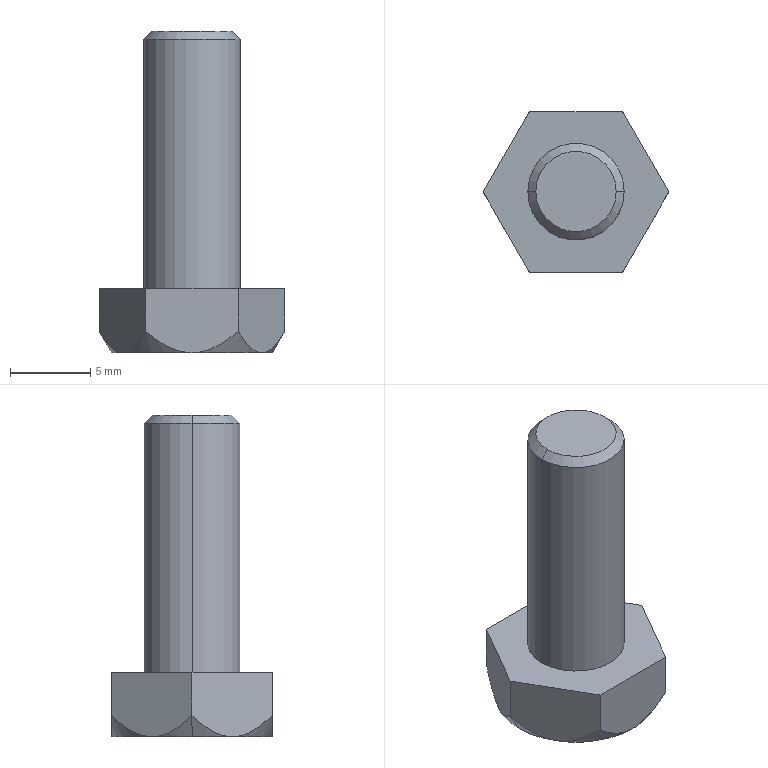Part | SolidWorks | features ICE 2, Chamfer 1, Extrusion 1 | 1 solid | 20 faces | box 11.547 x 10 x 20 mm | volume 793.318 mm3 | cone 9 | plane 9 | cylinder 2 | commonest cylinder face diameters 6 x2
STEP:
#1=CARTESIAN_POINT('',(2.5,0.,20.));
#2=VERTEX_POINT('',#1);
#3=CARTESIAN_POINT('',(-2.5,0.,20.));
#4=VERTEX_POINT('',#3);
#5=CARTESIAN_POINT('',(0.,0.,20.));
#6=DIRECTION('',(0.,0.,1.));
#7=DIRECTION('',(1.,0.,0.));
#8=AXIS2_PLACEMENT_3D('',#5,#6,#7);
#9=CIRCLE('',#8,2.5);
#10=EDGE_CURVE('',#2,#4,#9,.T.);
#11=ORIENTED_EDGE('',*,*,#10,.F.);
#12=CARTESIAN_POINT('',(3.,0.,19.5));
#13=VERTEX_POINT('',#12);
#14=CARTESIAN_POINT('',(2.5,0.,20.));
#15=DIRECTION('',(0.7071,0.,-0.7071));
#16=VECTOR('',#15,1000.);
#17=LINE('',#14,#16);
#18=EDGE_CURVE('',#2,#13,#17,.T.);
#19=ORIENTED_EDGE('',*,*,#18,.T.);
#20=CARTESIAN_POINT('',(-3.,0.,19.5));
#21=VERTEX_POINT('',#20);
#22=CARTESIAN_POINT('',(0.,0.,19.5));
#23=DIRECTION('',(0.,0.,-1.));
#24=DIRECTION('',(1.,0.,0.));
#25=AXIS2_PLACEMENT_3D('',#22,#23,#24);
#26=CIRCLE('',#25,3.);
#27=EDGE_CURVE('',#21,#13,#26,.T.);
#28=ORIENTED_EDGE('',*,*,#27,.F.);
#29=CARTESIAN_POINT('',(-2.5,0.,20.));
#30=DIRECTION('',(-0.7071,0.,-0.7071));
#31=VECTOR('',#30,1000.);
#32=LINE('',#29,#31);
#33=EDGE_CURVE('',#4,#21,#32,.T.);
#34=ORIENTED_EDGE('',*,*,#33,.F.);
#35=EDGE_LOOP('',(#11,#19,#28,#34));
#36=FACE_OUTER_BOUND('',#35,.T.);
#37=CARTESIAN_POINT('',(0.,0.,20.));
#38=DIRECTION('',(0.,0.,-1.));
#39=DIRECTION('',(-1.,0.,0.));
#40=AXIS2_PLACEMENT_3D('',#37,#38,#39);
#41=CONICAL_SURFACE('',#40,2.5,0.7854);
#42=ADVANCED_FACE('',(#36),#41,.T.);
#43=ORIENTED_EDGE('',*,*,#27,.T.);
#44=CARTESIAN_POINT('',(3.,0.,4.));
#45=VERTEX_POINT('',#44);
#46=CARTESIAN_POINT('',(3.,0.,20.));
#47=DIRECTION('',(0.,0.,-1.));
#48=VECTOR('',#47,1000.);
#49=LINE('',#46,#48);
#50=EDGE_CURVE('',#13,#45,#49,.T.);
#51=ORIENTED_EDGE('',*,*,#50,.T.);
#52=CARTESIAN_POINT('',(-3.,0.,4.));
#53=VERTEX_POINT('',#52);
#54=CARTESIAN_POINT('',(0.,0.,4.));
#55=DIRECTION('',(0.,0.,1.));
#56=DIRECTION('',(1.,0.,0.));
#57=AXIS2_PLACEMENT_3D('',#54,#55,#56);
#58=CIRCLE('',#57,3.);
#59=EDGE_CURVE('',#45,#53,#58,.T.);
#60=ORIENTED_EDGE('',*,*,#59,.T.);
#61=CARTESIAN_POINT('',(-3.,0.,20.));
#62=DIRECTION('',(0.,0.,-1.));
#63=VECTOR('',#62,1000.);
#64=LINE('',#61,#63);
#65=EDGE_CURVE('',#21,#53,#64,.T.);
#66=ORIENTED_EDGE('',*,*,#65,.F.);
#67=EDGE_LOOP('',(#43,#51,#60,#66));
#68=FACE_OUTER_BOUND('',#67,.T.);
#69=CARTESIAN_POINT('',(0.,0.,20.));
#70=DIRECTION('',(0.,0.,-1.));
#71=DIRECTION('',(-1.,0.,0.));
#72=AXIS2_PLACEMENT_3D('',#69,#70,#71);
#73=CYLINDRICAL_SURFACE('',#72,3.);
#74=ADVANCED_FACE('',(#68),#73,.T.);
#75=CARTESIAN_POINT('',(-4.33,2.5,0.));
#76=VERTEX_POINT('',#75);
#77=CARTESIAN_POINT('',(-5.,0.,0.));
#78=VERTEX_POINT('',#77);
#79=CARTESIAN_POINT('',(0.,0.,0.));
#80=DIRECTION('',(0.,0.,1.));
#81=DIRECTION('',(1.,0.,0.));
#82=AXIS2_PLACEMENT_3D('',#79,#80,#81);
#83=CIRCLE('',#82,5.);
#84=EDGE_CURVE('',#76,#78,#83,.T.);
#85=ORIENTED_EDGE('',*,*,#84,.T.);
#86=CARTESIAN_POINT('',(-5.774,0.,1.34));
#87=VERTEX_POINT('',#86);
#88=CARTESIAN_POINT('',(-5.,0.,0.));
#89=DIRECTION('',(-0.5,0.,0.866));
#90=VECTOR('',#89,1000.);
#91=LINE('',#88,#90);
#92=EDGE_CURVE('',#78,#87,#91,.T.);
#93=ORIENTED_EDGE('',*,*,#92,.T.);
#94=CARTESIAN_POINT('',(-5.774,0.,1.34));
#95=CARTESIAN_POINT('',(-5.568,0.3557,0.9841));
#96=CARTESIAN_POINT('',(-5.352,0.7302,0.6615));
#97=CARTESIAN_POINT('',(-4.991,1.355,0.2887));
#98=CARTESIAN_POINT('',(-4.864,1.576,0.1837));
#99=CARTESIAN_POINT('',(-4.668,1.915,0.07581));
#100=CARTESIAN_POINT('',(-4.602,2.03,0.0478));
#101=CARTESIAN_POINT('',(-4.467,2.263,0.009812));
#102=CARTESIAN_POINT('',(-4.398,2.383,0.));
#103=CARTESIAN_POINT('',(-4.33,2.5,0.));
#104=B_SPLINE_CURVE_WITH_KNOTS('',3,(#94,#95,#96,#97,#98,#99,#100,#101,#102,#103),.UNSPECIFIED.,.F.,.F.,(4,2,2,2,4),(0.000000303,0.001616,0.002424,0.002828,0.003232),.UNSPECIFIED.);
#105=EDGE_CURVE('',#87,#76,#104,.T.);
#106=ORIENTED_EDGE('',*,*,#105,.T.);
#107=EDGE_LOOP('',(#85,#93,#106));
#108=FACE_OUTER_BOUND('',#107,.T.);
#109=CARTESIAN_POINT('',(0.,0.,0.));
#110=DIRECTION('',(0.,0.,1.));
#111=DIRECTION('',(-1.,0.,0.));
#112=AXIS2_PLACEMENT_3D('',#109,#110,#111);
#113=CONICAL_SURFACE('',#112,5.,0.5236);
#114=ADVANCED_FACE('',(#108),#113,.T.);
#115=CARTESIAN_POINT('',(2.887,5.,1.34));
#116=VERTEX_POINT('',#115);
#117=CARTESIAN_POINT('',(4.33,2.5,0.));
#118=VERTEX_POINT('',#117);
#119=CARTESIAN_POINT('',(2.887,5.,1.34));
#120=CARTESIAN_POINT('',(3.092,4.644,0.9841));
#121=CARTESIAN_POINT('',(3.308,4.27,0.6615));
#122=CARTESIAN_POINT('',(3.669,3.645,0.2887));
#123=CARTESIAN_POINT('',(3.797,3.424,0.1837));
#124=CARTESIAN_POINT('',(3.992,3.085,0.07581));
#125=CARTESIAN_POINT('',(4.059,2.97,0.0478));
#126=CARTESIAN_POINT('',(4.193,2.737,0.009812));
#127=CARTESIAN_POINT('',(4.262,2.617,0.));
#128=CARTESIAN_POINT('',(4.33,2.5,0.));
#129=B_SPLINE_CURVE_WITH_KNOTS('',3,(#119,#120,#121,#122,#123,#124,#125,#126,#127,#128),.UNSPECIFIED.,.F.,.F.,(4,2,2,2,4),(0.000000303,0.001616,0.002424,0.002828,0.003232),.UNSPECIFIED.);
#130=EDGE_CURVE('',#116,#118,#129,.T.);
#131=ORIENTED_EDGE('',*,*,#130,.F.);
#132=CARTESIAN_POINT('',(2.887,5.,4.));
#133=VERTEX_POINT('',#132);
#134=CARTESIAN_POINT('',(2.887,5.,4.));
#135=DIRECTION('',(0.,0.,-1.));
#136=VECTOR('',#135,1000.);
#137=LINE('',#134,#136);
#138=EDGE_CURVE('',#133,#116,#137,.T.);
#139=ORIENTED_EDGE('',*,*,#138,.F.);
#140=CARTESIAN_POINT('',(5.774,0.,4.));
#141=VERTEX_POINT('',#140);
#142=CARTESIAN_POINT('',(5.774,0.,4.));
#143=DIRECTION('',(-0.5,0.866,0.));
#144=VECTOR('',#143,1000.);
#145=LINE('',#142,#144);
#146=EDGE_CURVE('',#141,#133,#145,.T.);
#147=ORIENTED_EDGE('',*,*,#146,.F.);
#148=CARTESIAN_POINT('',(5.774,0.,1.34));
#149=VERTEX_POINT('',#148);
#150=CARTESIAN_POINT('',(5.774,0.,4.));
#151=DIRECTION('',(0.,0.,-1.));
#152=VECTOR('',#151,1000.);
#153=LINE('',#150,#152);
#154=EDGE_CURVE('',#141,#149,#153,.T.);
#155=ORIENTED_EDGE('',*,*,#154,.T.);
#156=CARTESIAN_POINT('',(4.33,2.5,0.));
#157=CARTESIAN_POINT('',(4.466,2.265,0.));
#158=CARTESIAN_POINT('',(4.599,2.034,0.0383));
#159=CARTESIAN_POINT('',(4.863,1.578,0.1827));
#160=CARTESIAN_POINT('',(4.988,1.361,0.2859));
#161=CARTESIAN_POINT('',(5.228,0.9455,0.5326));
#162=CARTESIAN_POINT('',(5.343,0.7456,0.6772));
#163=CARTESIAN_POINT('',(5.565,0.3618,0.9919));
#164=CARTESIAN_POINT('',(5.671,0.1781,1.162));
#165=CARTESIAN_POINT('',(5.774,0.,1.34));
#166=B_SPLINE_CURVE_WITH_KNOTS('',3,(#156,#157,#158,#159,#160,#161,#162,#163,#164,#165),.UNSPECIFIED.,.F.,.F.,(4,2,2,2,4),(0.003232,0.004038,0.004845,0.005652,0.006458),.UNSPECIFIED.);
#167=EDGE_CURVE('',#118,#149,#166,.T.);
#168=ORIENTED_EDGE('',*,*,#167,.F.);
#169=EDGE_LOOP('',(#131,#139,#147,#155,#168));
#170=FACE_OUTER_BOUND('',#169,.T.);
#171=CARTESIAN_POINT('',(5.774,0.,4.));
#172=DIRECTION('',(-0.866,-0.5,0.));
#173=DIRECTION('',(0.5,-0.866,0.));
#174=AXIS2_PLACEMENT_3D('',#171,#172,#173);
#175=PLANE('',#174);
#176=ADVANCED_FACE('',(#170),#175,.F.);
#177=CARTESIAN_POINT('',(-2.887,5.,1.34));
#178=VERTEX_POINT('',#177);
#179=CARTESIAN_POINT('',(0.,5.,0.));
#180=VERTEX_POINT('',#179);
#181=CARTESIAN_POINT('',(-2.887,5.,1.34));
#182=CARTESIAN_POINT('',(-2.683,5.,1.163));
#183=CARTESIAN_POINT('',(-2.472,5.,0.9945));
#184=CARTESIAN_POINT('',(-2.031,5.,0.6804));
#185=CARTESIAN_POINT('',(-1.798,5.,0.5344));
#186=CARTESIAN_POINT('',(-1.316,5.,0.286));
#187=CARTESIAN_POINT('',(-1.063,5.,0.1822));
#188=CARTESIAN_POINT('',(-0.5366,5.,0.03808));
#189=CARTESIAN_POINT('',(-0.2701,5.,0.));
#190=CARTESIAN_POINT('',(0.,5.,0.));
#191=B_SPLINE_CURVE_WITH_KNOTS('',3,(#181,#182,#183,#184,#185,#186,#187,#188,#189,#190),.UNSPECIFIED.,.F.,.F.,(4,2,2,2,4),(0.01162,0.01244,0.01325,0.01406,0.01487),.UNSPECIFIED.);
#192=EDGE_CURVE('',#178,#180,#191,.T.);
#193=ORIENTED_EDGE('',*,*,#192,.F.);
#194=CARTESIAN_POINT('',(-2.887,5.,4.));
#195=VERTEX_POINT('',#194);
#196=CARTESIAN_POINT('',(-2.887,5.,4.));
#197=DIRECTION('',(0.,0.,-1.));
#198=VECTOR('',#197,1000.);
#199=LINE('',#196,#198);
#200=EDGE_CURVE('',#195,#178,#199,.T.);
#201=ORIENTED_EDGE('',*,*,#200,.F.);
#202=CARTESIAN_POINT('',(2.887,5.,4.));
#203=DIRECTION('',(-1.,0.,0.));
#204=VECTOR('',#203,1000.);
#205=LINE('',#202,#204);
#206=EDGE_CURVE('',#133,#195,#205,.T.);
#207=ORIENTED_EDGE('',*,*,#206,.F.);
#208=ORIENTED_EDGE('',*,*,#138,.T.);
#209=CARTESIAN_POINT('',(0.,5.,0.));
#210=CARTESIAN_POINT('',(0.2696,5.,0.));
#211=CARTESIAN_POINT('',(0.5439,5.,0.03965));
#212=CARTESIAN_POINT('',(1.066,5.,0.1833));
#213=CARTESIAN_POINT('',(1.32,5.,0.2879));
#214=CARTESIAN_POINT('',(2.042,5.,0.6607));
#215=CARTESIAN_POINT('',(2.477,5.,0.9847));
#216=CARTESIAN_POINT('',(2.887,5.,1.34));
#217=B_SPLINE_CURVE_WITH_KNOTS('',3,(#209,#210,#211,#212,#213,#214,#215,#216),.UNSPECIFIED.,.F.,.F.,(4,2,2,4),(0.01487,0.01568,0.01649,0.01812),.UNSPECIFIED.);
#218=EDGE_CURVE('',#180,#116,#217,.T.);
#219=ORIENTED_EDGE('',*,*,#218,.F.);
#220=EDGE_LOOP('',(#193,#201,#207,#208,#219));
#221=FACE_OUTER_BOUND('',#220,.T.);
#222=CARTESIAN_POINT('',(2.887,5.,4.));
#223=DIRECTION('',(0.,-1.,0.));
#224=DIRECTION('',(1.,0.,0.));
#225=AXIS2_PLACEMENT_3D('',#222,#223,#224);
#226=PLANE('',#225);
#227=ADVANCED_FACE('',(#221),#226,.F.);
#228=ORIENTED_EDGE('',*,*,#105,.F.);
#229=CARTESIAN_POINT('',(-5.774,0.,4.));
#230=VERTEX_POINT('',#229);
#231=CARTESIAN_POINT('',(-5.774,0.,4.));
#232=DIRECTION('',(0.,0.,-1.));
#233=VECTOR('',#232,1000.);
#234=LINE('',#231,#233);
#235=EDGE_CURVE('',#230,#87,#234,.T.);
#236=ORIENTED_EDGE('',*,*,#235,.F.);
#237=CARTESIAN_POINT('',(-2.887,5.,4.));
#238=DIRECTION('',(-0.5,-0.866,0.));
#239=VECTOR('',#238,1000.);
#240=LINE('',#237,#239);
#241=EDGE_CURVE('',#195,#230,#240,.T.);
#242=ORIENTED_EDGE('',*,*,#241,.F.);
#243=ORIENTED_EDGE('',*,*,#200,.T.);
#244=CARTESIAN_POINT('',(-4.33,2.5,0.));
#245=CARTESIAN_POINT('',(-4.195,2.735,0.));
#246=CARTESIAN_POINT('',(-4.061,2.966,0.0383));
#247=CARTESIAN_POINT('',(-3.798,3.422,0.1827));
#248=CARTESIAN_POINT('',(-3.672,3.639,0.2859));
#249=CARTESIAN_POINT('',(-3.433,4.055,0.5326));
#250=CARTESIAN_POINT('',(-3.317,4.254,0.6772));
#251=CARTESIAN_POINT('',(-3.096,4.638,0.9919));
#252=CARTESIAN_POINT('',(-2.99,4.822,1.162));
#253=CARTESIAN_POINT('',(-2.887,5.,1.34));
#254=B_SPLINE_CURVE_WITH_KNOTS('',3,(#244,#245,#246,#247,#248,#249,#250,#251,#252,#253),.UNSPECIFIED.,.F.,.F.,(4,2,2,2,4),(0.003232,0.004038,0.004845,0.005652,0.006458),.UNSPECIFIED.);
#255=EDGE_CURVE('',#76,#178,#254,.T.);
#256=ORIENTED_EDGE('',*,*,#255,.F.);
#257=EDGE_LOOP('',(#228,#236,#242,#243,#256));
#258=FACE_OUTER_BOUND('',#257,.T.);
#259=CARTESIAN_POINT('',(-2.887,5.,4.));
#260=DIRECTION('',(0.866,-0.5,0.));
#261=DIRECTION('',(0.5,0.866,0.));
#262=AXIS2_PLACEMENT_3D('',#259,#260,#261);
#263=PLANE('',#262);
#264=ADVANCED_FACE('',(#258),#263,.F.);
#265=CARTESIAN_POINT('',(-2.887,-5.,1.34));
#266=VERTEX_POINT('',#265);
#267=CARTESIAN_POINT('',(-4.33,-2.5,0.));
#268=VERTEX_POINT('',#267);
#269=CARTESIAN_POINT('',(-2.887,-5.,1.34));
#270=CARTESIAN_POINT('',(-3.092,-4.644,0.9841));
#271=CARTESIAN_POINT('',(-3.308,-4.27,0.6615));
#272=CARTESIAN_POINT('',(-3.669,-3.645,0.2887));
#273=CARTESIAN_POINT('',(-3.797,-3.424,0.1837));
#274=CARTESIAN_POINT('',(-3.992,-3.085,0.07581));
#275=CARTESIAN_POINT('',(-4.059,-2.97,0.0478));
#276=CARTESIAN_POINT('',(-4.193,-2.737,0.009812));
#277=CARTESIAN_POINT('',(-4.262,-2.617,0.));
#278=CARTESIAN_POINT('',(-4.33,-2.5,0.));
#279=B_SPLINE_CURVE_WITH_KNOTS('',3,(#269,#270,#271,#272,#273,#274,#275,#276,#277,#278),.UNSPECIFIED.,.F.,.F.,(4,2,2,2,4),(0.000000303,0.001616,0.002424,0.002828,0.003232),.UNSPECIFIED.);
#280=EDGE_CURVE('',#266,#268,#279,.T.);
#281=ORIENTED_EDGE('',*,*,#280,.F.);
#282=CARTESIAN_POINT('',(-2.887,-5.,4.));
#283=VERTEX_POINT('',#282);
#284=CARTESIAN_POINT('',(-2.887,-5.,4.));
#285=DIRECTION('',(0.,0.,-1.));
#286=VECTOR('',#285,1000.);
#287=LINE('',#284,#286);
#288=EDGE_CURVE('',#283,#266,#287,.T.);
#289=ORIENTED_EDGE('',*,*,#288,.F.);
#290=CARTESIAN_POINT('',(-5.774,0.,4.));
#291=DIRECTION('',(0.5,-0.866,0.));
#292=VECTOR('',#291,1000.);
#293=LINE('',#290,#292);
#294=EDGE_CURVE('',#230,#283,#293,.T.);
#295=ORIENTED_EDGE('',*,*,#294,.F.);
#296=ORIENTED_EDGE('',*,*,#235,.T.);
#297=CARTESIAN_POINT('',(-4.33,-2.5,0.));
#298=CARTESIAN_POINT('',(-4.466,-2.265,0.));
#299=CARTESIAN_POINT('',(-4.599,-2.034,0.0383));
#300=CARTESIAN_POINT('',(-4.863,-1.578,0.1827));
#301=CARTESIAN_POINT('',(-4.988,-1.361,0.2859));
#302=CARTESIAN_POINT('',(-5.228,-0.9455,0.5326));
#303=CARTESIAN_POINT('',(-5.343,-0.7456,0.6772));
#304=CARTESIAN_POINT('',(-5.565,-0.3618,0.9919));
#305=CARTESIAN_POINT('',(-5.671,-0.1781,1.162));
#306=CARTESIAN_POINT('',(-5.774,0.,1.34));
#307=B_SPLINE_CURVE_WITH_KNOTS('',3,(#297,#298,#299,#300,#301,#302,#303,#304,#305,#306),.UNSPECIFIED.,.F.,.F.,(4,2,2,2,4),(0.003232,0.004038,0.004845,0.005652,0.006458),.UNSPECIFIED.);
#308=EDGE_CURVE('',#268,#87,#307,.T.);
#309=ORIENTED_EDGE('',*,*,#308,.F.);
#310=EDGE_LOOP('',(#281,#289,#295,#296,#309));
#311=FACE_OUTER_BOUND('',#310,.T.);
#312=CARTESIAN_POINT('',(-5.774,0.,4.));
#313=DIRECTION('',(0.866,0.5,0.));
#314=DIRECTION('',(-0.5,0.866,0.));
#315=AXIS2_PLACEMENT_3D('',#312,#313,#314);
#316=PLANE('',#315);
#317=ADVANCED_FACE('',(#311),#316,.F.);
#318=CARTESIAN_POINT('',(2.887,-5.,1.34));
#319=VERTEX_POINT('',#318);
#320=CARTESIAN_POINT('',(0.,-5.,0.));
#321=VERTEX_POINT('',#320);
#322=CARTESIAN_POINT('',(2.887,-5.,1.34));
#323=CARTESIAN_POINT('',(2.683,-5.,1.163));
#324=CARTESIAN_POINT('',(2.472,-5.,0.9945));
#325=CARTESIAN_POINT('',(2.031,-5.,0.6804));
#326=CARTESIAN_POINT('',(1.798,-5.,0.5344));
#327=CARTESIAN_POINT('',(1.316,-5.,0.286));
#328=CARTESIAN_POINT('',(1.063,-5.,0.1822));
#329=CARTESIAN_POINT('',(0.5366,-5.,0.03808));
#330=CARTESIAN_POINT('',(0.2701,-5.,0.));
#331=CARTESIAN_POINT('',(0.,-5.,0.));
#332=B_SPLINE_CURVE_WITH_KNOTS('',3,(#322,#323,#324,#325,#326,#327,#328,#329,#330,#331),.UNSPECIFIED.,.F.,.F.,(4,2,2,2,4),(0.01162,0.01244,0.01325,0.01406,0.01487),.UNSPECIFIED.);
#333=EDGE_CURVE('',#319,#321,#332,.T.);
#334=ORIENTED_EDGE('',*,*,#333,.F.);
#335=CARTESIAN_POINT('',(2.887,-5.,4.));
#336=VERTEX_POINT('',#335);
#337=CARTESIAN_POINT('',(2.887,-5.,4.));
#338=DIRECTION('',(0.,0.,-1.));
#339=VECTOR('',#338,1000.);
#340=LINE('',#337,#339);
#341=EDGE_CURVE('',#336,#319,#340,.T.);
#342=ORIENTED_EDGE('',*,*,#341,.F.);
#343=CARTESIAN_POINT('',(-2.887,-5.,4.));
#344=DIRECTION('',(1.,0.,0.));
#345=VECTOR('',#344,1000.);
#346=LINE('',#343,#345);
#347=EDGE_CURVE('',#283,#336,#346,.T.);
#348=ORIENTED_EDGE('',*,*,#347,.F.);
#349=ORIENTED_EDGE('',*,*,#288,.T.);
#350=CARTESIAN_POINT('',(0.,-5.,0.));
#351=CARTESIAN_POINT('',(-0.2696,-5.,0.));
#352=CARTESIAN_POINT('',(-0.5439,-5.,0.03965));
#353=CARTESIAN_POINT('',(-1.066,-5.,0.1833));
#354=CARTESIAN_POINT('',(-1.32,-5.,0.2879));
#355=CARTESIAN_POINT('',(-2.042,-5.,0.6607));
#356=CARTESIAN_POINT('',(-2.477,-5.,0.9847));
#357=CARTESIAN_POINT('',(-2.887,-5.,1.34));
#358=B_SPLINE_CURVE_WITH_KNOTS('',3,(#350,#351,#352,#353,#354,#355,#356,#357),.UNSPECIFIED.,.F.,.F.,(4,2,2,4),(0.01487,0.01568,0.01649,0.01812),.UNSPECIFIED.);
#359=EDGE_CURVE('',#321,#266,#358,.T.);
#360=ORIENTED_EDGE('',*,*,#359,.F.);
#361=EDGE_LOOP('',(#334,#342,#348,#349,#360));
#362=FACE_OUTER_BOUND('',#361,.T.);
#363=CARTESIAN_POINT('',(-2.887,-5.,4.));
#364=DIRECTION('',(0.,1.,0.));
#365=DIRECTION('',(0.,0.,1.));
#366=AXIS2_PLACEMENT_3D('',#363,#364,#365);
#367=PLANE('',#366);
#368=ADVANCED_FACE('',(#362),#367,.F.);
#369=CARTESIAN_POINT('',(4.33,-2.5,0.));
#370=VERTEX_POINT('',#369);
#371=CARTESIAN_POINT('',(5.774,0.,1.34));
#372=CARTESIAN_POINT('',(5.568,-0.3557,0.9841));
#373=CARTESIAN_POINT('',(5.352,-0.7302,0.6615));
#374=CARTESIAN_POINT('',(4.991,-1.355,0.2887));
#375=CARTESIAN_POINT('',(4.864,-1.576,0.1837));
#376=CARTESIAN_POINT('',(4.668,-1.915,0.07581));
#377=CARTESIAN_POINT('',(4.602,-2.03,0.0478));
#378=CARTESIAN_POINT('',(4.467,-2.263,0.009812));
#379=CARTESIAN_POINT('',(4.398,-2.383,0.));
#380=CARTESIAN_POINT('',(4.33,-2.5,0.));
#381=B_SPLINE_CURVE_WITH_KNOTS('',3,(#371,#372,#373,#374,#375,#376,#377,#378,#379,#380),.UNSPECIFIED.,.F.,.F.,(4,2,2,2,4),(0.000000303,0.001616,0.002424,0.002828,0.003232),.UNSPECIFIED.);
#382=EDGE_CURVE('',#149,#370,#381,.T.);
#383=ORIENTED_EDGE('',*,*,#382,.F.);
#384=ORIENTED_EDGE('',*,*,#154,.F.);
#385=CARTESIAN_POINT('',(2.887,-5.,4.));
#386=DIRECTION('',(0.5,0.866,0.));
#387=VECTOR('',#386,1000.);
#388=LINE('',#385,#387);
#389=EDGE_CURVE('',#336,#141,#388,.T.);
#390=ORIENTED_EDGE('',*,*,#389,.F.);
#391=ORIENTED_EDGE('',*,*,#341,.T.);
#392=CARTESIAN_POINT('',(4.33,-2.5,0.));
#393=CARTESIAN_POINT('',(4.195,-2.735,0.));
#394=CARTESIAN_POINT('',(4.061,-2.966,0.0383));
#395=CARTESIAN_POINT('',(3.798,-3.422,0.1827));
#396=CARTESIAN_POINT('',(3.672,-3.639,0.2859));
#397=CARTESIAN_POINT('',(3.433,-4.055,0.5326));
#398=CARTESIAN_POINT('',(3.317,-4.254,0.6772));
#399=CARTESIAN_POINT('',(3.096,-4.638,0.9919));
#400=CARTESIAN_POINT('',(2.99,-4.822,1.162));
#401=CARTESIAN_POINT('',(2.887,-5.,1.34));
#402=B_SPLINE_CURVE_WITH_KNOTS('',3,(#392,#393,#394,#395,#396,#397,#398,#399,#400,#401),.UNSPECIFIED.,.F.,.F.,(4,2,2,2,4),(0.003232,0.004038,0.004845,0.005652,0.006458),.UNSPECIFIED.);
#403=EDGE_CURVE('',#370,#319,#402,.T.);
#404=ORIENTED_EDGE('',*,*,#403,.F.);
#405=EDGE_LOOP('',(#383,#384,#390,#391,#404));
#406=FACE_OUTER_BOUND('',#405,.T.);
#407=CARTESIAN_POINT('',(2.887,-5.,4.));
#408=DIRECTION('',(-0.866,0.5,0.));
#409=DIRECTION('',(-0.5,-0.866,0.));
#410=AXIS2_PLACEMENT_3D('',#407,#408,#409);
#411=PLANE('',#410);
#412=ADVANCED_FACE('',(#406),#411,.F.);
#413=CARTESIAN_POINT('',(0.,0.,4.));
#414=DIRECTION('',(0.,0.,1.));
#415=DIRECTION('',(1.,0.,0.));
#416=AXIS2_PLACEMENT_3D('',#413,#414,#415);
#417=CIRCLE('',#416,3.);
#418=EDGE_CURVE('',#53,#45,#417,.T.);
#419=ORIENTED_EDGE('',*,*,#418,.F.);
#420=ORIENTED_EDGE('',*,*,#59,.F.);
#421=EDGE_LOOP('',(#419,#420));
#422=FACE_BOUND('',#421,.T.);
#423=ORIENTED_EDGE('',*,*,#146,.T.);
#424=ORIENTED_EDGE('',*,*,#206,.T.);
#425=ORIENTED_EDGE('',*,*,#241,.T.);
#426=ORIENTED_EDGE('',*,*,#294,.T.);
#427=ORIENTED_EDGE('',*,*,#347,.T.);
#428=ORIENTED_EDGE('',*,*,#389,.T.);
#429=EDGE_LOOP('',(#423,#424,#425,#426,#427,#428));
#430=FACE_OUTER_BOUND('',#429,.T.);
#431=CARTESIAN_POINT('',(0.,0.,4.));
#432=DIRECTION('',(0.,0.,1.));
#433=DIRECTION('',(1.,0.,0.));
#434=AXIS2_PLACEMENT_3D('',#431,#432,#433);
#435=PLANE('',#434);
#436=ADVANCED_FACE('',(#422,#430),#435,.T.);
#437=ORIENTED_EDGE('',*,*,#167,.T.);
#438=ORIENTED_EDGE('',*,*,#382,.T.);
#439=CARTESIAN_POINT('',(0.,0.,0.));
#440=DIRECTION('',(0.,0.,1.));
#441=DIRECTION('',(1.,0.,0.));
#442=AXIS2_PLACEMENT_3D('',#439,#440,#441);
#443=CIRCLE('',#442,5.);
#444=EDGE_CURVE('',#370,#118,#443,.T.);
#445=ORIENTED_EDGE('',*,*,#444,.T.);
#446=EDGE_LOOP('',(#437,#438,#445));
#447=FACE_OUTER_BOUND('',#446,.T.);
#448=CARTESIAN_POINT('',(0.,0.,0.));
#449=DIRECTION('',(0.,0.,1.));
#450=DIRECTION('',(-1.,0.,0.));
#451=AXIS2_PLACEMENT_3D('',#448,#449,#450);
#452=CONICAL_SURFACE('',#451,5.,0.5236);
#453=ADVANCED_FACE('',(#447),#452,.T.);
#454=ORIENTED_EDGE('',*,*,#333,.T.);
#455=CARTESIAN_POINT('',(0.,0.,0.));
#456=DIRECTION('',(0.,0.,1.));
#457=DIRECTION('',(1.,0.,0.));
#458=AXIS2_PLACEMENT_3D('',#455,#456,#457);
#459=CIRCLE('',#458,5.);
#460=EDGE_CURVE('',#321,#370,#459,.T.);
#461=ORIENTED_EDGE('',*,*,#460,.T.);
#462=ORIENTED_EDGE('',*,*,#403,.T.);
#463=EDGE_LOOP('',(#454,#461,#462));
#464=FACE_OUTER_BOUND('',#463,.T.);
#465=CARTESIAN_POINT('',(0.,0.,0.));
#466=DIRECTION('',(0.,0.,1.));
#467=DIRECTION('',(-1.,0.,0.));
#468=AXIS2_PLACEMENT_3D('',#465,#466,#467);
#469=CONICAL_SURFACE('',#468,5.,0.5236);
#470=ADVANCED_FACE('',(#464),#469,.T.);
#471=ORIENTED_EDGE('',*,*,#280,.T.);
#472=CARTESIAN_POINT('',(0.,0.,0.));
#473=DIRECTION('',(0.,0.,1.));
#474=DIRECTION('',(1.,0.,0.));
#475=AXIS2_PLACEMENT_3D('',#472,#473,#474);
#476=CIRCLE('',#475,5.);
#477=EDGE_CURVE('',#268,#321,#476,.T.);
#478=ORIENTED_EDGE('',*,*,#477,.T.);
#479=ORIENTED_EDGE('',*,*,#359,.T.);
#480=EDGE_LOOP('',(#471,#478,#479));
#481=FACE_OUTER_BOUND('',#480,.T.);
#482=CARTESIAN_POINT('',(0.,0.,0.));
#483=DIRECTION('',(0.,0.,1.));
#484=DIRECTION('',(-1.,0.,0.));
#485=AXIS2_PLACEMENT_3D('',#482,#483,#484);
#486=CONICAL_SURFACE('',#485,5.,0.5236);
#487=ADVANCED_FACE('',(#481),#486,.T.);
#488=ORIENTED_EDGE('',*,*,#92,.F.);
#489=CARTESIAN_POINT('',(0.,0.,0.));
#490=DIRECTION('',(0.,0.,1.));
#491=DIRECTION('',(1.,0.,0.));
#492=AXIS2_PLACEMENT_3D('',#489,#490,#491);
#493=CIRCLE('',#492,5.);
#494=EDGE_CURVE('',#78,#268,#493,.T.);
#495=ORIENTED_EDGE('',*,*,#494,.T.);
#496=ORIENTED_EDGE('',*,*,#308,.T.);
#497=EDGE_LOOP('',(#488,#495,#496));
#498=FACE_OUTER_BOUND('',#497,.T.);
#499=CARTESIAN_POINT('',(0.,0.,0.));
#500=DIRECTION('',(0.,0.,1.));
#501=DIRECTION('',(-1.,0.,0.));
#502=AXIS2_PLACEMENT_3D('',#499,#500,#501);
#503=CONICAL_SURFACE('',#502,5.,0.5236);
#504=ADVANCED_FACE('',(#498),#503,.T.);
#505=ORIENTED_EDGE('',*,*,#255,.T.);
#506=ORIENTED_EDGE('',*,*,#192,.T.);
#507=CARTESIAN_POINT('',(0.,0.,0.));
#508=DIRECTION('',(0.,0.,-1.));
#509=DIRECTION('',(-1.,0.,0.));
#510=AXIS2_PLACEMENT_3D('',#507,#508,#509);
#511=CIRCLE('',#510,5.);
#512=EDGE_CURVE('',#76,#180,#511,.T.);
#513=ORIENTED_EDGE('',*,*,#512,.F.);
#514=EDGE_LOOP('',(#505,#506,#513));
#515=FACE_OUTER_BOUND('',#514,.T.);
#516=CARTESIAN_POINT('',(0.,0.,0.));
#517=DIRECTION('',(0.,0.,1.));
#518=DIRECTION('',(-1.,0.,0.));
#519=AXIS2_PLACEMENT_3D('',#516,#517,#518);
#520=CONICAL_SURFACE('',#519,5.,0.5236);
#521=ADVANCED_FACE('',(#515),#520,.T.);
#522=ORIENTED_EDGE('',*,*,#218,.T.);
#523=ORIENTED_EDGE('',*,*,#130,.T.);
#524=CARTESIAN_POINT('',(0.,0.,0.));
#525=DIRECTION('',(0.,0.,1.));
#526=DIRECTION('',(1.,0.,0.));
#527=AXIS2_PLACEMENT_3D('',#524,#525,#526);
#528=CIRCLE('',#527,5.);
#529=EDGE_CURVE('',#118,#180,#528,.T.);
#530=ORIENTED_EDGE('',*,*,#529,.T.);
#531=EDGE_LOOP('',(#522,#523,#530));
#532=FACE_OUTER_BOUND('',#531,.T.);
#533=CARTESIAN_POINT('',(0.,0.,0.));
#534=DIRECTION('',(0.,0.,1.));
#535=DIRECTION('',(-1.,0.,0.));
#536=AXIS2_PLACEMENT_3D('',#533,#534,#535);
#537=CONICAL_SURFACE('',#536,5.,0.5236);
#538=ADVANCED_FACE('',(#532),#537,.T.);
#539=ORIENTED_EDGE('',*,*,#529,.F.);
#540=ORIENTED_EDGE('',*,*,#444,.F.);
#541=ORIENTED_EDGE('',*,*,#460,.F.);
#542=ORIENTED_EDGE('',*,*,#477,.F.);
#543=ORIENTED_EDGE('',*,*,#494,.F.);
#544=ORIENTED_EDGE('',*,*,#84,.F.);
#545=ORIENTED_EDGE('',*,*,#512,.T.);
#546=EDGE_LOOP('',(#539,#540,#541,#542,#543,#544,#545));
#547=FACE_OUTER_BOUND('',#546,.T.);
#548=CARTESIAN_POINT('',(0.,0.,0.));
#549=DIRECTION('',(0.,0.,1.));
#550=DIRECTION('',(1.,0.,0.));
#551=AXIS2_PLACEMENT_3D('',#548,#549,#550);
#552=PLANE('',#551);
#553=ADVANCED_FACE('',(#547),#552,.F.);
#554=ORIENTED_EDGE('',*,*,#50,.F.);
#555=CARTESIAN_POINT('',(0.,0.,19.5));
#556=DIRECTION('',(0.,0.,-1.));
#557=DIRECTION('',(1.,0.,0.));
#558=AXIS2_PLACEMENT_3D('',#555,#556,#557);
#559=CIRCLE('',#558,3.);
#560=EDGE_CURVE('',#13,#21,#559,.T.);
#561=ORIENTED_EDGE('',*,*,#560,.T.);
#562=ORIENTED_EDGE('',*,*,#65,.T.);
#563=ORIENTED_EDGE('',*,*,#418,.T.);
#564=EDGE_LOOP('',(#554,#561,#562,#563));
#565=FACE_OUTER_BOUND('',#564,.T.);
#566=CARTESIAN_POINT('',(0.,0.,20.));
#567=DIRECTION('',(0.,0.,-1.));
#568=DIRECTION('',(-1.,0.,0.));
#569=AXIS2_PLACEMENT_3D('',#566,#567,#568);
#570=CYLINDRICAL_SURFACE('',#569,3.);
#571=ADVANCED_FACE('',(#565),#570,.T.);
#572=CARTESIAN_POINT('',(0.,0.,20.));
#573=DIRECTION('',(0.,0.,1.));
#574=DIRECTION('',(1.,0.,0.));
#575=AXIS2_PLACEMENT_3D('',#572,#573,#574);
#576=CIRCLE('',#575,2.5);
#577=EDGE_CURVE('',#4,#2,#576,.T.);
#578=ORIENTED_EDGE('',*,*,#577,.T.);
#579=ORIENTED_EDGE('',*,*,#10,.T.);
#580=EDGE_LOOP('',(#578,#579));
#581=FACE_OUTER_BOUND('',#580,.T.);
#582=CARTESIAN_POINT('',(0.,0.,20.));
#583=DIRECTION('',(0.,0.,1.));
#584=DIRECTION('',(1.,0.,0.));
#585=AXIS2_PLACEMENT_3D('',#582,#583,#584);
#586=PLANE('',#585);
#587=ADVANCED_FACE('',(#581),#586,.T.);
#588=ORIENTED_EDGE('',*,*,#18,.F.);
#589=ORIENTED_EDGE('',*,*,#577,.F.);
#590=ORIENTED_EDGE('',*,*,#33,.T.);
#591=ORIENTED_EDGE('',*,*,#560,.F.);
#592=EDGE_LOOP('',(#588,#589,#590,#591));
#593=FACE_OUTER_BOUND('',#592,.T.);
#594=CARTESIAN_POINT('',(0.,0.,20.));
#595=DIRECTION('',(0.,0.,-1.));
#596=DIRECTION('',(-1.,0.,0.));
#597=AXIS2_PLACEMENT_3D('',#594,#595,#596);
#598=CONICAL_SURFACE('',#597,2.5,0.7854);
#599=ADVANCED_FACE('',(#593),#598,.T.);
#600=CLOSED_SHELL('',(#42,#74,#114,#176,#227,#264,#317,#368,#412,#436,#453,#470,#487,#504,#521,#538,#553,#571,#587,#599));
#601=MANIFOLD_SOLID_BREP('',#600);
#602=CARTESIAN_POINT('',(0.,0.,0.));
#603=DIRECTION('',(0.,0.,1.));
#604=DIRECTION('',(1.,0.,0.));
#605=AXIS2_PLACEMENT_3D('',#602,#603,#604);
#606=(LENGTH_UNIT()NAMED_UNIT(*)SI_UNIT(.MILLI.,.METRE.));
#607=UNCERTAINTY_MEASURE_WITH_UNIT(LENGTH_MEASURE(0.00001),#606,'','');
#608=(NAMED_UNIT(*)PLANE_ANGLE_UNIT()SI_UNIT($,.RADIAN.));
#609=(NAMED_UNIT(*)SI_UNIT($,.STERADIAN.)SOLID_ANGLE_UNIT());
#610=(GEOMETRIC_REPRESENTATION_CONTEXT(3)GLOBAL_UNCERTAINTY_ASSIGNED_CONTEXT((#607))GLOBAL_UNIT_ASSIGNED_CONTEXT((#606,#608,#609))REPRESENTATION_CONTEXT('',''));
#611=ADVANCED_BREP_SHAPE_REPRESENTATION('',(#601,#605),#610);